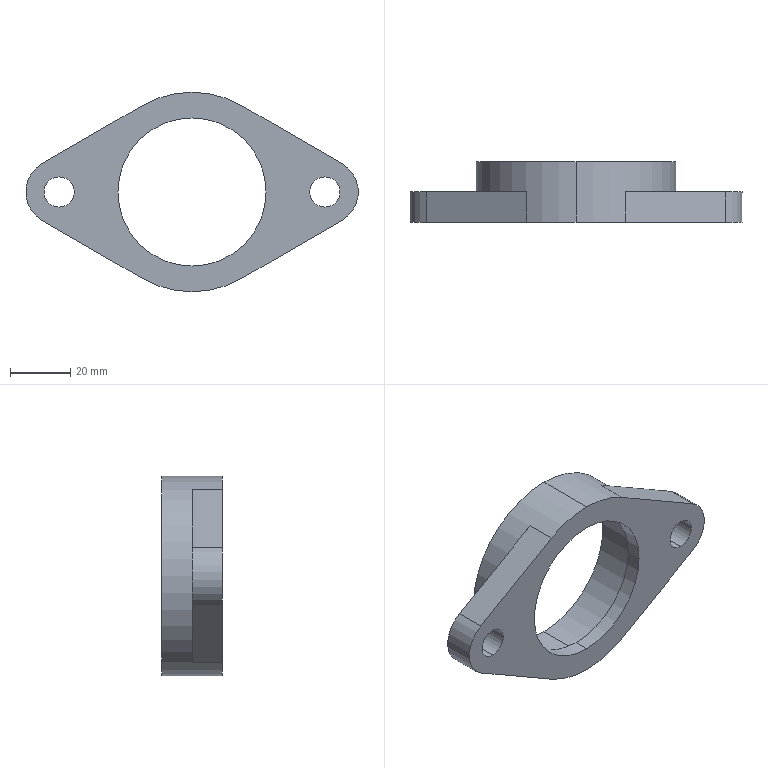Part | SolidWorks | features ICE 3, Extrusion 1 | 1 solid | 21 faces | box 110 x 20 x 66 mm | volume 35046 mm3 | cylinder 12 | plane 9 | commonest cylinder face diameters 10 x4 22 x2 49 x2 55 x2 66 x2
STEP:
#1=CARTESIAN_POINT('',(0.,0.,-24.5));
#2=VERTEX_POINT('',#1);
#3=CARTESIAN_POINT('',(0.,0.,24.5));
#4=VERTEX_POINT('',#3);
#5=CARTESIAN_POINT('',(0.,0.,0.));
#6=DIRECTION('',(0.,1.,0.));
#7=DIRECTION('',(0.,0.,1.));
#8=AXIS2_PLACEMENT_3D('',#5,#6,#7);
#9=CIRCLE('',#8,24.5);
#10=EDGE_CURVE('',#2,#4,#9,.T.);
#11=ORIENTED_EDGE('',*,*,#10,.F.);
#12=CARTESIAN_POINT('',(0.,5.,-24.5));
#13=VERTEX_POINT('',#12);
#14=CARTESIAN_POINT('',(0.,-10.,-24.5));
#15=DIRECTION('',(0.,1.,0.));
#16=VECTOR('',#15,1000.);
#17=LINE('',#14,#16);
#18=EDGE_CURVE('',#2,#13,#17,.T.);
#19=ORIENTED_EDGE('',*,*,#18,.T.);
#20=CARTESIAN_POINT('',(0.,5.,24.5));
#21=VERTEX_POINT('',#20);
#22=CARTESIAN_POINT('',(0.,5.,0.));
#23=DIRECTION('',(0.,1.,0.));
#24=DIRECTION('',(0.,0.,1.));
#25=AXIS2_PLACEMENT_3D('',#22,#23,#24);
#26=CIRCLE('',#25,24.5);
#27=EDGE_CURVE('',#13,#21,#26,.T.);
#28=ORIENTED_EDGE('',*,*,#27,.T.);
#29=CARTESIAN_POINT('',(0.,-10.,24.5));
#30=DIRECTION('',(0.,1.,0.));
#31=VECTOR('',#30,1000.);
#32=LINE('',#29,#31);
#33=EDGE_CURVE('',#4,#21,#32,.T.);
#34=ORIENTED_EDGE('',*,*,#33,.F.);
#35=EDGE_LOOP('',(#11,#19,#28,#34));
#36=FACE_OUTER_BOUND('',#35,.T.);
#37=CARTESIAN_POINT('',(0.,-10.,0.));
#38=DIRECTION('',(0.,1.,0.));
#39=DIRECTION('',(0.,0.,1.));
#40=AXIS2_PLACEMENT_3D('',#37,#38,#39);
#41=CYLINDRICAL_SURFACE('',#40,24.5);
#42=ADVANCED_FACE('',(#36),#41,.F.);
#43=CARTESIAN_POINT('',(0.,5.,-27.5));
#44=VERTEX_POINT('',#43);
#45=CARTESIAN_POINT('',(0.,5.,27.5));
#46=VERTEX_POINT('',#45);
#47=CARTESIAN_POINT('',(0.,5.,0.));
#48=DIRECTION('',(0.,1.,0.));
#49=DIRECTION('',(0.,0.,1.));
#50=AXIS2_PLACEMENT_3D('',#47,#48,#49);
#51=CIRCLE('',#50,27.5);
#52=EDGE_CURVE('',#44,#46,#51,.T.);
#53=ORIENTED_EDGE('',*,*,#52,.F.);
#54=CARTESIAN_POINT('',(0.,20.,-27.5));
#55=VERTEX_POINT('',#54);
#56=CARTESIAN_POINT('',(0.,5.,-27.5));
#57=DIRECTION('',(0.,1.,0.));
#58=VECTOR('',#57,1000.);
#59=LINE('',#56,#58);
#60=EDGE_CURVE('',#44,#55,#59,.T.);
#61=ORIENTED_EDGE('',*,*,#60,.T.);
#62=CARTESIAN_POINT('',(0.,20.,27.5));
#63=VERTEX_POINT('',#62);
#64=CARTESIAN_POINT('',(0.,20.,0.));
#65=DIRECTION('',(0.,1.,0.));
#66=DIRECTION('',(0.,0.,1.));
#67=AXIS2_PLACEMENT_3D('',#64,#65,#66);
#68=CIRCLE('',#67,27.5);
#69=EDGE_CURVE('',#55,#63,#68,.T.);
#70=ORIENTED_EDGE('',*,*,#69,.T.);
#71=CARTESIAN_POINT('',(0.,5.,27.5));
#72=DIRECTION('',(0.,1.,0.));
#73=VECTOR('',#72,1000.);
#74=LINE('',#71,#73);
#75=EDGE_CURVE('',#46,#63,#74,.T.);
#76=ORIENTED_EDGE('',*,*,#75,.F.);
#77=EDGE_LOOP('',(#53,#61,#70,#76));
#78=FACE_OUTER_BOUND('',#77,.T.);
#79=CARTESIAN_POINT('',(0.,5.,0.));
#80=DIRECTION('',(0.,1.,0.));
#81=DIRECTION('',(0.,0.,1.));
#82=AXIS2_PLACEMENT_3D('',#79,#80,#81);
#83=CYLINDRICAL_SURFACE('',#82,27.5);
#84=ADVANCED_FACE('',(#78),#83,.F.);
#85=CARTESIAN_POINT('',(44.,10.,-5.));
#86=VERTEX_POINT('',#85);
#87=CARTESIAN_POINT('',(44.,10.,5.));
#88=VERTEX_POINT('',#87);
#89=CARTESIAN_POINT('',(44.,10.,0.));
#90=DIRECTION('',(0.,1.,0.));
#91=DIRECTION('',(0.,0.,1.));
#92=AXIS2_PLACEMENT_3D('',#89,#90,#91);
#93=CIRCLE('',#92,5.);
#94=EDGE_CURVE('',#86,#88,#93,.T.);
#95=ORIENTED_EDGE('',*,*,#94,.T.);
#96=CARTESIAN_POINT('',(44.,0.,5.));
#97=VERTEX_POINT('',#96);
#98=CARTESIAN_POINT('',(44.,10.,5.));
#99=DIRECTION('',(0.,-1.,0.));
#100=VECTOR('',#99,1000.);
#101=LINE('',#98,#100);
#102=EDGE_CURVE('',#88,#97,#101,.T.);
#103=ORIENTED_EDGE('',*,*,#102,.T.);
#104=CARTESIAN_POINT('',(44.,0.,-5.));
#105=VERTEX_POINT('',#104);
#106=CARTESIAN_POINT('',(44.,0.,0.));
#107=DIRECTION('',(0.,1.,0.));
#108=DIRECTION('',(0.,0.,1.));
#109=AXIS2_PLACEMENT_3D('',#106,#107,#108);
#110=CIRCLE('',#109,5.);
#111=EDGE_CURVE('',#105,#97,#110,.T.);
#112=ORIENTED_EDGE('',*,*,#111,.F.);
#113=CARTESIAN_POINT('',(44.,10.,-5.));
#114=DIRECTION('',(0.,-1.,0.));
#115=VECTOR('',#114,1000.);
#116=LINE('',#113,#115);
#117=EDGE_CURVE('',#86,#105,#116,.T.);
#118=ORIENTED_EDGE('',*,*,#117,.F.);
#119=EDGE_LOOP('',(#95,#103,#112,#118));
#120=FACE_OUTER_BOUND('',#119,.T.);
#121=CARTESIAN_POINT('',(44.,10.,0.));
#122=DIRECTION('',(0.,-1.,0.));
#123=DIRECTION('',(0.,0.,-1.));
#124=AXIS2_PLACEMENT_3D('',#121,#122,#123);
#125=CYLINDRICAL_SURFACE('',#124,5.);
#126=ADVANCED_FACE('',(#120),#125,.F.);
#127=CARTESIAN_POINT('',(-44.,10.,-5.));
#128=VERTEX_POINT('',#127);
#129=CARTESIAN_POINT('',(-44.,10.,5.));
#130=VERTEX_POINT('',#129);
#131=CARTESIAN_POINT('',(-44.,10.,0.));
#132=DIRECTION('',(0.,1.,0.));
#133=DIRECTION('',(0.,0.,1.));
#134=AXIS2_PLACEMENT_3D('',#131,#132,#133);
#135=CIRCLE('',#134,5.);
#136=EDGE_CURVE('',#128,#130,#135,.T.);
#137=ORIENTED_EDGE('',*,*,#136,.T.);
#138=CARTESIAN_POINT('',(-44.,0.,5.));
#139=VERTEX_POINT('',#138);
#140=CARTESIAN_POINT('',(-44.,10.,5.));
#141=DIRECTION('',(0.,-1.,0.));
#142=VECTOR('',#141,1000.);
#143=LINE('',#140,#142);
#144=EDGE_CURVE('',#130,#139,#143,.T.);
#145=ORIENTED_EDGE('',*,*,#144,.T.);
#146=CARTESIAN_POINT('',(-44.,0.,-5.));
#147=VERTEX_POINT('',#146);
#148=CARTESIAN_POINT('',(-44.,0.,0.));
#149=DIRECTION('',(0.,1.,0.));
#150=DIRECTION('',(0.,0.,1.));
#151=AXIS2_PLACEMENT_3D('',#148,#149,#150);
#152=CIRCLE('',#151,5.);
#153=EDGE_CURVE('',#147,#139,#152,.T.);
#154=ORIENTED_EDGE('',*,*,#153,.F.);
#155=CARTESIAN_POINT('',(-44.,10.,-5.));
#156=DIRECTION('',(0.,-1.,0.));
#157=VECTOR('',#156,1000.);
#158=LINE('',#155,#157);
#159=EDGE_CURVE('',#128,#147,#158,.T.);
#160=ORIENTED_EDGE('',*,*,#159,.F.);
#161=EDGE_LOOP('',(#137,#145,#154,#160));
#162=FACE_OUTER_BOUND('',#161,.T.);
#163=CARTESIAN_POINT('',(-44.,10.,0.));
#164=DIRECTION('',(0.,-1.,0.));
#165=DIRECTION('',(0.,0.,-1.));
#166=AXIS2_PLACEMENT_3D('',#163,#164,#165);
#167=CYLINDRICAL_SURFACE('',#166,5.);
#168=ADVANCED_FACE('',(#162),#167,.F.);
#169=CARTESIAN_POINT('',(0.,20.,33.));
#170=VERTEX_POINT('',#169);
#171=CARTESIAN_POINT('',(0.,20.,-33.));
#172=VERTEX_POINT('',#171);
#173=CARTESIAN_POINT('',(0.,20.,0.));
#174=DIRECTION('',(0.,1.,0.));
#175=DIRECTION('',(0.,0.,1.));
#176=AXIS2_PLACEMENT_3D('',#173,#174,#175);
#177=CIRCLE('',#176,33.);
#178=EDGE_CURVE('',#170,#172,#177,.T.);
#179=ORIENTED_EDGE('',*,*,#178,.F.);
#180=CARTESIAN_POINT('',(0.,0.,33.));
#181=VERTEX_POINT('',#180);
#182=CARTESIAN_POINT('',(0.,10.,33.));
#183=DIRECTION('',(0.,-1.,0.));
#184=VECTOR('',#183,1000.);
#185=LINE('',#182,#184);
#186=EDGE_CURVE('',#170,#181,#185,.T.);
#187=ORIENTED_EDGE('',*,*,#186,.T.);
#188=CARTESIAN_POINT('',(16.5,0.,28.579));
#189=VERTEX_POINT('',#188);
#190=CARTESIAN_POINT('',(0.,0.,0.));
#191=DIRECTION('',(0.,1.,0.));
#192=DIRECTION('',(0.,0.,1.));
#193=AXIS2_PLACEMENT_3D('',#190,#191,#192);
#194=CIRCLE('',#193,33.);
#195=EDGE_CURVE('',#181,#189,#194,.T.);
#196=ORIENTED_EDGE('',*,*,#195,.T.);
#197=CARTESIAN_POINT('',(16.5,10.,28.579));
#198=VERTEX_POINT('',#197);
#199=CARTESIAN_POINT('',(16.5,10.,28.579));
#200=DIRECTION('',(0.,-1.,0.));
#201=VECTOR('',#200,1000.);
#202=LINE('',#199,#201);
#203=EDGE_CURVE('',#198,#189,#202,.T.);
#204=ORIENTED_EDGE('',*,*,#203,.F.);
#205=CARTESIAN_POINT('',(16.5,10.,-28.579));
#206=VERTEX_POINT('',#205);
#207=CARTESIAN_POINT('',(0.,10.,0.));
#208=DIRECTION('',(0.,1.,0.));
#209=DIRECTION('',(0.,0.,1.));
#210=AXIS2_PLACEMENT_3D('',#207,#208,#209);
#211=CIRCLE('',#210,33.);
#212=EDGE_CURVE('',#198,#206,#211,.T.);
#213=ORIENTED_EDGE('',*,*,#212,.T.);
#214=CARTESIAN_POINT('',(16.5,0.,-28.579));
#215=VERTEX_POINT('',#214);
#216=CARTESIAN_POINT('',(16.5,10.,-28.579));
#217=DIRECTION('',(0.,-1.,0.));
#218=VECTOR('',#217,1000.);
#219=LINE('',#216,#218);
#220=EDGE_CURVE('',#206,#215,#219,.T.);
#221=ORIENTED_EDGE('',*,*,#220,.T.);
#222=CARTESIAN_POINT('',(0.,0.,-33.));
#223=VERTEX_POINT('',#222);
#224=CARTESIAN_POINT('',(0.,0.,0.));
#225=DIRECTION('',(0.,1.,0.));
#226=DIRECTION('',(0.,0.,1.));
#227=AXIS2_PLACEMENT_3D('',#224,#225,#226);
#228=CIRCLE('',#227,33.);
#229=EDGE_CURVE('',#215,#223,#228,.T.);
#230=ORIENTED_EDGE('',*,*,#229,.T.);
#231=CARTESIAN_POINT('',(0.,10.,-33.));
#232=DIRECTION('',(0.,-1.,0.));
#233=VECTOR('',#232,1000.);
#234=LINE('',#231,#233);
#235=EDGE_CURVE('',#172,#223,#234,.T.);
#236=ORIENTED_EDGE('',*,*,#235,.F.);
#237=EDGE_LOOP('',(#179,#187,#196,#204,#213,#221,#230,#236));
#238=FACE_OUTER_BOUND('',#237,.T.);
#239=CARTESIAN_POINT('',(0.,10.,0.));
#240=DIRECTION('',(0.,-1.,0.));
#241=DIRECTION('',(0.,0.,-1.));
#242=AXIS2_PLACEMENT_3D('',#239,#240,#241);
#243=CYLINDRICAL_SURFACE('',#242,33.);
#244=ADVANCED_FACE('',(#238),#243,.T.);
#245=ORIENTED_EDGE('',*,*,#212,.F.);
#246=CARTESIAN_POINT('',(49.5,10.,9.526));
#247=VERTEX_POINT('',#246);
#248=CARTESIAN_POINT('',(49.5,10.,9.526));
#249=DIRECTION('',(0.866,0.,-0.5));
#250=VECTOR('',#249,1000.);
#251=LINE('',#248,#250);
#252=EDGE_CURVE('',#198,#247,#251,.T.);
#253=ORIENTED_EDGE('',*,*,#252,.T.);
#254=CARTESIAN_POINT('',(49.5,10.,-9.526));
#255=VERTEX_POINT('',#254);
#256=CARTESIAN_POINT('',(44.,10.,0.));
#257=DIRECTION('',(0.,1.,0.));
#258=DIRECTION('',(0.,0.,1.));
#259=AXIS2_PLACEMENT_3D('',#256,#257,#258);
#260=CIRCLE('',#259,11.);
#261=EDGE_CURVE('',#247,#255,#260,.T.);
#262=ORIENTED_EDGE('',*,*,#261,.T.);
#263=CARTESIAN_POINT('',(16.5,10.,-28.579));
#264=DIRECTION('',(-0.866,0.,-0.5));
#265=VECTOR('',#264,1000.);
#266=LINE('',#263,#265);
#267=EDGE_CURVE('',#255,#206,#266,.T.);
#268=ORIENTED_EDGE('',*,*,#267,.T.);
#269=EDGE_LOOP('',(#245,#253,#262,#268));
#270=FACE_OUTER_BOUND('',#269,.T.);
#271=ORIENTED_EDGE('',*,*,#94,.F.);
#272=CARTESIAN_POINT('',(44.,10.,0.));
#273=DIRECTION('',(0.,1.,0.));
#274=DIRECTION('',(0.,0.,1.));
#275=AXIS2_PLACEMENT_3D('',#272,#273,#274);
#276=CIRCLE('',#275,5.);
#277=EDGE_CURVE('',#88,#86,#276,.T.);
#278=ORIENTED_EDGE('',*,*,#277,.F.);
#279=EDGE_LOOP('',(#271,#278));
#280=FACE_BOUND('',#279,.T.);
#281=CARTESIAN_POINT('',(-44.,10.,0.));
#282=DIRECTION('',(0.,1.,0.));
#283=DIRECTION('',(0.,0.,1.));
#284=AXIS2_PLACEMENT_3D('',#281,#282,#283);
#285=PLANE('',#284);
#286=ADVANCED_FACE('',(#270,#280),#285,.T.);
#287=CARTESIAN_POINT('',(-16.5,10.,-28.579));
#288=VERTEX_POINT('',#287);
#289=CARTESIAN_POINT('',(-16.5,10.,28.579));
#290=VERTEX_POINT('',#289);
#291=CARTESIAN_POINT('',(0.,10.,0.));
#292=DIRECTION('',(0.,1.,0.));
#293=DIRECTION('',(0.,0.,1.));
#294=AXIS2_PLACEMENT_3D('',#291,#292,#293);
#295=CIRCLE('',#294,33.);
#296=EDGE_CURVE('',#288,#290,#295,.T.);
#297=ORIENTED_EDGE('',*,*,#296,.F.);
#298=CARTESIAN_POINT('',(-49.5,10.,-9.526));
#299=VERTEX_POINT('',#298);
#300=CARTESIAN_POINT('',(-49.5,10.,-9.526));
#301=DIRECTION('',(-0.866,0.,0.5));
#302=VECTOR('',#301,1000.);
#303=LINE('',#300,#302);
#304=EDGE_CURVE('',#288,#299,#303,.T.);
#305=ORIENTED_EDGE('',*,*,#304,.T.);
#306=CARTESIAN_POINT('',(-49.5,10.,9.526));
#307=VERTEX_POINT('',#306);
#308=CARTESIAN_POINT('',(-44.,10.,0.));
#309=DIRECTION('',(0.,1.,0.));
#310=DIRECTION('',(0.,0.,1.));
#311=AXIS2_PLACEMENT_3D('',#308,#309,#310);
#312=CIRCLE('',#311,11.);
#313=EDGE_CURVE('',#299,#307,#312,.T.);
#314=ORIENTED_EDGE('',*,*,#313,.T.);
#315=CARTESIAN_POINT('',(-16.5,10.,28.579));
#316=DIRECTION('',(0.866,0.,0.5));
#317=VECTOR('',#316,1000.);
#318=LINE('',#315,#317);
#319=EDGE_CURVE('',#307,#290,#318,.T.);
#320=ORIENTED_EDGE('',*,*,#319,.T.);
#321=EDGE_LOOP('',(#297,#305,#314,#320));
#322=FACE_OUTER_BOUND('',#321,.T.);
#323=ORIENTED_EDGE('',*,*,#136,.F.);
#324=CARTESIAN_POINT('',(-44.,10.,0.));
#325=DIRECTION('',(0.,1.,0.));
#326=DIRECTION('',(0.,0.,1.));
#327=AXIS2_PLACEMENT_3D('',#324,#325,#326);
#328=CIRCLE('',#327,5.);
#329=EDGE_CURVE('',#130,#128,#328,.T.);
#330=ORIENTED_EDGE('',*,*,#329,.F.);
#331=EDGE_LOOP('',(#323,#330));
#332=FACE_BOUND('',#331,.T.);
#333=CARTESIAN_POINT('',(-44.,10.,0.));
#334=DIRECTION('',(0.,1.,0.));
#335=DIRECTION('',(0.,0.,1.));
#336=AXIS2_PLACEMENT_3D('',#333,#334,#335);
#337=PLANE('',#336);
#338=ADVANCED_FACE('',(#322,#332),#337,.T.);
#339=CARTESIAN_POINT('',(0.,0.,0.));
#340=DIRECTION('',(0.,1.,0.));
#341=DIRECTION('',(0.,0.,1.));
#342=AXIS2_PLACEMENT_3D('',#339,#340,#341);
#343=CIRCLE('',#342,24.5);
#344=EDGE_CURVE('',#4,#2,#343,.T.);
#345=ORIENTED_EDGE('',*,*,#344,.T.);
#346=ORIENTED_EDGE('',*,*,#10,.T.);
#347=EDGE_LOOP('',(#345,#346));
#348=FACE_BOUND('',#347,.T.);
#349=ORIENTED_EDGE('',*,*,#153,.T.);
#350=CARTESIAN_POINT('',(-44.,0.,0.));
#351=DIRECTION('',(0.,1.,0.));
#352=DIRECTION('',(0.,0.,1.));
#353=AXIS2_PLACEMENT_3D('',#350,#351,#352);
#354=CIRCLE('',#353,5.);
#355=EDGE_CURVE('',#139,#147,#354,.T.);
#356=ORIENTED_EDGE('',*,*,#355,.T.);
#357=EDGE_LOOP('',(#349,#356));
#358=FACE_BOUND('',#357,.T.);
#359=CARTESIAN_POINT('',(-49.5,0.,-9.526));
#360=VERTEX_POINT('',#359);
#361=CARTESIAN_POINT('',(-49.5,0.,9.526));
#362=VERTEX_POINT('',#361);
#363=CARTESIAN_POINT('',(-44.,0.,0.));
#364=DIRECTION('',(0.,1.,0.));
#365=DIRECTION('',(0.,0.,1.));
#366=AXIS2_PLACEMENT_3D('',#363,#364,#365);
#367=CIRCLE('',#366,11.);
#368=EDGE_CURVE('',#360,#362,#367,.T.);
#369=ORIENTED_EDGE('',*,*,#368,.F.);
#370=CARTESIAN_POINT('',(-16.5,0.,-28.579));
#371=VERTEX_POINT('',#370);
#372=CARTESIAN_POINT('',(-49.5,0.,-9.526));
#373=DIRECTION('',(-0.866,0.,0.5));
#374=VECTOR('',#373,1000.);
#375=LINE('',#372,#374);
#376=EDGE_CURVE('',#371,#360,#375,.T.);
#377=ORIENTED_EDGE('',*,*,#376,.F.);
#378=CARTESIAN_POINT('',(0.,0.,0.));
#379=DIRECTION('',(0.,1.,0.));
#380=DIRECTION('',(0.,0.,1.));
#381=AXIS2_PLACEMENT_3D('',#378,#379,#380);
#382=CIRCLE('',#381,33.);
#383=EDGE_CURVE('',#223,#371,#382,.T.);
#384=ORIENTED_EDGE('',*,*,#383,.F.);
#385=ORIENTED_EDGE('',*,*,#229,.F.);
#386=CARTESIAN_POINT('',(49.5,0.,-9.526));
#387=VERTEX_POINT('',#386);
#388=CARTESIAN_POINT('',(16.5,0.,-28.579));
#389=DIRECTION('',(-0.866,0.,-0.5));
#390=VECTOR('',#389,1000.);
#391=LINE('',#388,#390);
#392=EDGE_CURVE('',#387,#215,#391,.T.);
#393=ORIENTED_EDGE('',*,*,#392,.F.);
#394=CARTESIAN_POINT('',(49.5,0.,9.526));
#395=VERTEX_POINT('',#394);
#396=CARTESIAN_POINT('',(44.,0.,0.));
#397=DIRECTION('',(0.,1.,0.));
#398=DIRECTION('',(0.,0.,1.));
#399=AXIS2_PLACEMENT_3D('',#396,#397,#398);
#400=CIRCLE('',#399,11.);
#401=EDGE_CURVE('',#395,#387,#400,.T.);
#402=ORIENTED_EDGE('',*,*,#401,.F.);
#403=CARTESIAN_POINT('',(49.5,0.,9.526));
#404=DIRECTION('',(0.866,0.,-0.5));
#405=VECTOR('',#404,1000.);
#406=LINE('',#403,#405);
#407=EDGE_CURVE('',#189,#395,#406,.T.);
#408=ORIENTED_EDGE('',*,*,#407,.F.);
#409=ORIENTED_EDGE('',*,*,#195,.F.);
#410=CARTESIAN_POINT('',(-16.5,0.,28.579));
#411=VERTEX_POINT('',#410);
#412=CARTESIAN_POINT('',(0.,0.,0.));
#413=DIRECTION('',(0.,1.,0.));
#414=DIRECTION('',(0.,0.,1.));
#415=AXIS2_PLACEMENT_3D('',#412,#413,#414);
#416=CIRCLE('',#415,33.);
#417=EDGE_CURVE('',#411,#181,#416,.T.);
#418=ORIENTED_EDGE('',*,*,#417,.F.);
#419=CARTESIAN_POINT('',(-16.5,0.,28.579));
#420=DIRECTION('',(0.866,0.,0.5));
#421=VECTOR('',#420,1000.);
#422=LINE('',#419,#421);
#423=EDGE_CURVE('',#362,#411,#422,.T.);
#424=ORIENTED_EDGE('',*,*,#423,.F.);
#425=EDGE_LOOP('',(#369,#377,#384,#385,#393,#402,#408,#409,#418,#424));
#426=FACE_OUTER_BOUND('',#425,.T.);
#427=ORIENTED_EDGE('',*,*,#111,.T.);
#428=CARTESIAN_POINT('',(44.,0.,0.));
#429=DIRECTION('',(0.,1.,0.));
#430=DIRECTION('',(0.,0.,1.));
#431=AXIS2_PLACEMENT_3D('',#428,#429,#430);
#432=CIRCLE('',#431,5.);
#433=EDGE_CURVE('',#97,#105,#432,.T.);
#434=ORIENTED_EDGE('',*,*,#433,.T.);
#435=EDGE_LOOP('',(#427,#434));
#436=FACE_BOUND('',#435,.T.);
#437=CARTESIAN_POINT('',(-44.,0.,0.));
#438=DIRECTION('',(0.,1.,0.));
#439=DIRECTION('',(0.,0.,1.));
#440=AXIS2_PLACEMENT_3D('',#437,#438,#439);
#441=PLANE('',#440);
#442=ADVANCED_FACE('',(#348,#358,#426,#436),#441,.F.);
#443=ORIENTED_EDGE('',*,*,#368,.T.);
#444=CARTESIAN_POINT('',(-49.5,10.,9.526));
#445=DIRECTION('',(0.,-1.,0.));
#446=VECTOR('',#445,1000.);
#447=LINE('',#444,#446);
#448=EDGE_CURVE('',#307,#362,#447,.T.);
#449=ORIENTED_EDGE('',*,*,#448,.F.);
#450=ORIENTED_EDGE('',*,*,#313,.F.);
#451=CARTESIAN_POINT('',(-49.5,10.,-9.526));
#452=DIRECTION('',(0.,-1.,0.));
#453=VECTOR('',#452,1000.);
#454=LINE('',#451,#453);
#455=EDGE_CURVE('',#299,#360,#454,.T.);
#456=ORIENTED_EDGE('',*,*,#455,.T.);
#457=EDGE_LOOP('',(#443,#449,#450,#456));
#458=FACE_OUTER_BOUND('',#457,.T.);
#459=CARTESIAN_POINT('',(-44.,10.,0.));
#460=DIRECTION('',(0.,-1.,0.));
#461=DIRECTION('',(0.,0.,-1.));
#462=AXIS2_PLACEMENT_3D('',#459,#460,#461);
#463=CYLINDRICAL_SURFACE('',#462,11.);
#464=ADVANCED_FACE('',(#458),#463,.T.);
#465=ORIENTED_EDGE('',*,*,#423,.T.);
#466=CARTESIAN_POINT('',(-16.5,10.,28.579));
#467=DIRECTION('',(0.,-1.,0.));
#468=VECTOR('',#467,1000.);
#469=LINE('',#466,#468);
#470=EDGE_CURVE('',#290,#411,#469,.T.);
#471=ORIENTED_EDGE('',*,*,#470,.F.);
#472=ORIENTED_EDGE('',*,*,#319,.F.);
#473=ORIENTED_EDGE('',*,*,#448,.T.);
#474=EDGE_LOOP('',(#465,#471,#472,#473));
#475=FACE_OUTER_BOUND('',#474,.T.);
#476=CARTESIAN_POINT('',(-16.5,10.,28.579));
#477=DIRECTION('',(0.5,0.,-0.866));
#478=DIRECTION('',(-0.866,0.,-0.5));
#479=AXIS2_PLACEMENT_3D('',#476,#477,#478);
#480=PLANE('',#479);
#481=ADVANCED_FACE('',(#475),#480,.F.);
#482=ORIENTED_EDGE('',*,*,#407,.T.);
#483=CARTESIAN_POINT('',(49.5,10.,9.526));
#484=DIRECTION('',(0.,-1.,0.));
#485=VECTOR('',#484,1000.);
#486=LINE('',#483,#485);
#487=EDGE_CURVE('',#247,#395,#486,.T.);
#488=ORIENTED_EDGE('',*,*,#487,.F.);
#489=ORIENTED_EDGE('',*,*,#252,.F.);
#490=ORIENTED_EDGE('',*,*,#203,.T.);
#491=EDGE_LOOP('',(#482,#488,#489,#490));
#492=FACE_OUTER_BOUND('',#491,.T.);
#493=CARTESIAN_POINT('',(49.5,10.,9.526));
#494=DIRECTION('',(-0.5,0.,-0.866));
#495=DIRECTION('',(-0.866,0.,0.5));
#496=AXIS2_PLACEMENT_3D('',#493,#494,#495);
#497=PLANE('',#496);
#498=ADVANCED_FACE('',(#492),#497,.F.);
#499=ORIENTED_EDGE('',*,*,#401,.T.);
#500=CARTESIAN_POINT('',(49.5,10.,-9.526));
#501=DIRECTION('',(0.,-1.,0.));
#502=VECTOR('',#501,1000.);
#503=LINE('',#500,#502);
#504=EDGE_CURVE('',#255,#387,#503,.T.);
#505=ORIENTED_EDGE('',*,*,#504,.F.);
#506=ORIENTED_EDGE('',*,*,#261,.F.);
#507=ORIENTED_EDGE('',*,*,#487,.T.);
#508=EDGE_LOOP('',(#499,#505,#506,#507));
#509=FACE_OUTER_BOUND('',#508,.T.);
#510=CARTESIAN_POINT('',(44.,10.,0.));
#511=DIRECTION('',(0.,-1.,0.));
#512=DIRECTION('',(0.,0.,-1.));
#513=AXIS2_PLACEMENT_3D('',#510,#511,#512);
#514=CYLINDRICAL_SURFACE('',#513,11.);
#515=ADVANCED_FACE('',(#509),#514,.T.);
#516=ORIENTED_EDGE('',*,*,#392,.T.);
#517=ORIENTED_EDGE('',*,*,#220,.F.);
#518=ORIENTED_EDGE('',*,*,#267,.F.);
#519=ORIENTED_EDGE('',*,*,#504,.T.);
#520=EDGE_LOOP('',(#516,#517,#518,#519));
#521=FACE_OUTER_BOUND('',#520,.T.);
#522=CARTESIAN_POINT('',(16.5,10.,-28.579));
#523=DIRECTION('',(-0.5,0.,0.866));
#524=DIRECTION('',(0.866,0.,0.5));
#525=AXIS2_PLACEMENT_3D('',#522,#523,#524);
#526=PLANE('',#525);
#527=ADVANCED_FACE('',(#521),#526,.F.);
#528=ORIENTED_EDGE('',*,*,#186,.F.);
#529=CARTESIAN_POINT('',(0.,20.,0.));
#530=DIRECTION('',(0.,1.,0.));
#531=DIRECTION('',(0.,0.,1.));
#532=AXIS2_PLACEMENT_3D('',#529,#530,#531);
#533=CIRCLE('',#532,33.);
#534=EDGE_CURVE('',#172,#170,#533,.T.);
#535=ORIENTED_EDGE('',*,*,#534,.F.);
#536=ORIENTED_EDGE('',*,*,#235,.T.);
#537=ORIENTED_EDGE('',*,*,#383,.T.);
#538=CARTESIAN_POINT('',(-16.5,10.,-28.579));
#539=DIRECTION('',(0.,-1.,0.));
#540=VECTOR('',#539,1000.);
#541=LINE('',#538,#540);
#542=EDGE_CURVE('',#288,#371,#541,.T.);
#543=ORIENTED_EDGE('',*,*,#542,.F.);
#544=ORIENTED_EDGE('',*,*,#296,.T.);
#545=ORIENTED_EDGE('',*,*,#470,.T.);
#546=ORIENTED_EDGE('',*,*,#417,.T.);
#547=EDGE_LOOP('',(#528,#535,#536,#537,#543,#544,#545,#546));
#548=FACE_OUTER_BOUND('',#547,.T.);
#549=CARTESIAN_POINT('',(0.,10.,0.));
#550=DIRECTION('',(0.,-1.,0.));
#551=DIRECTION('',(0.,0.,-1.));
#552=AXIS2_PLACEMENT_3D('',#549,#550,#551);
#553=CYLINDRICAL_SURFACE('',#552,33.);
#554=ADVANCED_FACE('',(#548),#553,.T.);
#555=ORIENTED_EDGE('',*,*,#376,.T.);
#556=ORIENTED_EDGE('',*,*,#455,.F.);
#557=ORIENTED_EDGE('',*,*,#304,.F.);
#558=ORIENTED_EDGE('',*,*,#542,.T.);
#559=EDGE_LOOP('',(#555,#556,#557,#558));
#560=FACE_OUTER_BOUND('',#559,.T.);
#561=CARTESIAN_POINT('',(-49.5,10.,-9.526));
#562=DIRECTION('',(0.5,0.,0.866));
#563=DIRECTION('',(0.866,0.,-0.5));
#564=AXIS2_PLACEMENT_3D('',#561,#562,#563);
#565=PLANE('',#564);
#566=ADVANCED_FACE('',(#560),#565,.F.);
#567=ORIENTED_EDGE('',*,*,#144,.F.);
#568=ORIENTED_EDGE('',*,*,#329,.T.);
#569=ORIENTED_EDGE('',*,*,#159,.T.);
#570=ORIENTED_EDGE('',*,*,#355,.F.);
#571=EDGE_LOOP('',(#567,#568,#569,#570));
#572=FACE_OUTER_BOUND('',#571,.T.);
#573=CARTESIAN_POINT('',(-44.,10.,0.));
#574=DIRECTION('',(0.,-1.,0.));
#575=DIRECTION('',(0.,0.,-1.));
#576=AXIS2_PLACEMENT_3D('',#573,#574,#575);
#577=CYLINDRICAL_SURFACE('',#576,5.);
#578=ADVANCED_FACE('',(#572),#577,.F.);
#579=ORIENTED_EDGE('',*,*,#102,.F.);
#580=ORIENTED_EDGE('',*,*,#277,.T.);
#581=ORIENTED_EDGE('',*,*,#117,.T.);
#582=ORIENTED_EDGE('',*,*,#433,.F.);
#583=EDGE_LOOP('',(#579,#580,#581,#582));
#584=FACE_OUTER_BOUND('',#583,.T.);
#585=CARTESIAN_POINT('',(44.,10.,0.));
#586=DIRECTION('',(0.,-1.,0.));
#587=DIRECTION('',(0.,0.,-1.));
#588=AXIS2_PLACEMENT_3D('',#585,#586,#587);
#589=CYLINDRICAL_SURFACE('',#588,5.);
#590=ADVANCED_FACE('',(#584),#589,.F.);
#591=CARTESIAN_POINT('',(0.,20.,0.));
#592=DIRECTION('',(0.,1.,0.));
#593=DIRECTION('',(0.,0.,1.));
#594=AXIS2_PLACEMENT_3D('',#591,#592,#593);
#595=CIRCLE('',#594,27.5);
#596=EDGE_CURVE('',#63,#55,#595,.T.);
#597=ORIENTED_EDGE('',*,*,#596,.F.);
#598=ORIENTED_EDGE('',*,*,#69,.F.);
#599=EDGE_LOOP('',(#597,#598));
#600=FACE_BOUND('',#599,.T.);
#601=ORIENTED_EDGE('',*,*,#534,.T.);
#602=ORIENTED_EDGE('',*,*,#178,.T.);
#603=EDGE_LOOP('',(#601,#602));
#604=FACE_OUTER_BOUND('',#603,.T.);
#605=CARTESIAN_POINT('',(0.,20.,0.));
#606=DIRECTION('',(0.,1.,0.));
#607=DIRECTION('',(0.,0.,1.));
#608=AXIS2_PLACEMENT_3D('',#605,#606,#607);
#609=PLANE('',#608);
#610=ADVANCED_FACE('',(#600,#604),#609,.T.);
#611=ORIENTED_EDGE('',*,*,#60,.F.);
#612=CARTESIAN_POINT('',(0.,5.,0.));
#613=DIRECTION('',(0.,1.,0.));
#614=DIRECTION('',(0.,0.,1.));
#615=AXIS2_PLACEMENT_3D('',#612,#613,#614);
#616=CIRCLE('',#615,27.5);
#617=EDGE_CURVE('',#46,#44,#616,.T.);
#618=ORIENTED_EDGE('',*,*,#617,.F.);
#619=ORIENTED_EDGE('',*,*,#75,.T.);
#620=ORIENTED_EDGE('',*,*,#596,.T.);
#621=EDGE_LOOP('',(#611,#618,#619,#620));
#622=FACE_OUTER_BOUND('',#621,.T.);
#623=CARTESIAN_POINT('',(0.,5.,0.));
#624=DIRECTION('',(0.,1.,0.));
#625=DIRECTION('',(0.,0.,1.));
#626=AXIS2_PLACEMENT_3D('',#623,#624,#625);
#627=CYLINDRICAL_SURFACE('',#626,27.5);
#628=ADVANCED_FACE('',(#622),#627,.F.);
#629=CARTESIAN_POINT('',(0.,5.,0.));
#630=DIRECTION('',(0.,1.,0.));
#631=DIRECTION('',(0.,0.,1.));
#632=AXIS2_PLACEMENT_3D('',#629,#630,#631);
#633=CIRCLE('',#632,24.5);
#634=EDGE_CURVE('',#21,#13,#633,.T.);
#635=ORIENTED_EDGE('',*,*,#634,.F.);
#636=ORIENTED_EDGE('',*,*,#27,.F.);
#637=EDGE_LOOP('',(#635,#636));
#638=FACE_BOUND('',#637,.T.);
#639=ORIENTED_EDGE('',*,*,#617,.T.);
#640=ORIENTED_EDGE('',*,*,#52,.T.);
#641=EDGE_LOOP('',(#639,#640));
#642=FACE_OUTER_BOUND('',#641,.T.);
#643=CARTESIAN_POINT('',(0.,5.,0.));
#644=DIRECTION('',(0.,1.,0.));
#645=DIRECTION('',(0.,0.,1.));
#646=AXIS2_PLACEMENT_3D('',#643,#644,#645);
#647=PLANE('',#646);
#648=ADVANCED_FACE('',(#638,#642),#647,.T.);
#649=ORIENTED_EDGE('',*,*,#18,.F.);
#650=ORIENTED_EDGE('',*,*,#344,.F.);
#651=ORIENTED_EDGE('',*,*,#33,.T.);
#652=ORIENTED_EDGE('',*,*,#634,.T.);
#653=EDGE_LOOP('',(#649,#650,#651,#652));
#654=FACE_OUTER_BOUND('',#653,.T.);
#655=CARTESIAN_POINT('',(0.,-10.,0.));
#656=DIRECTION('',(0.,1.,0.));
#657=DIRECTION('',(0.,0.,1.));
#658=AXIS2_PLACEMENT_3D('',#655,#656,#657);
#659=CYLINDRICAL_SURFACE('',#658,24.5);
#660=ADVANCED_FACE('',(#654),#659,.F.);
#661=CLOSED_SHELL('',(#42,#84,#126,#168,#244,#286,#338,#442,#464,#481,#498,#515,#527,#554,#566,#578,#590,#610,#628,#648,#660));
#662=MANIFOLD_SOLID_BREP('',#661);
#663=CARTESIAN_POINT('',(0.,0.,0.));
#664=DIRECTION('',(0.,0.,1.));
#665=DIRECTION('',(1.,0.,0.));
#666=AXIS2_PLACEMENT_3D('',#663,#664,#665);
#667=(LENGTH_UNIT()NAMED_UNIT(*)SI_UNIT(.MILLI.,.METRE.));
#668=UNCERTAINTY_MEASURE_WITH_UNIT(LENGTH_MEASURE(0.00001),#667,'','');
#669=(NAMED_UNIT(*)PLANE_ANGLE_UNIT()SI_UNIT($,.RADIAN.));
#670=(NAMED_UNIT(*)SI_UNIT($,.STERADIAN.)SOLID_ANGLE_UNIT());
#671=(GEOMETRIC_REPRESENTATION_CONTEXT(3)GLOBAL_UNCERTAINTY_ASSIGNED_CONTEXT((#668))GLOBAL_UNIT_ASSIGNED_CONTEXT((#667,#669,#670))REPRESENTATION_CONTEXT('',''));
#672=ADVANCED_BREP_SHAPE_REPRESENTATION('',(#662,#666),#671);